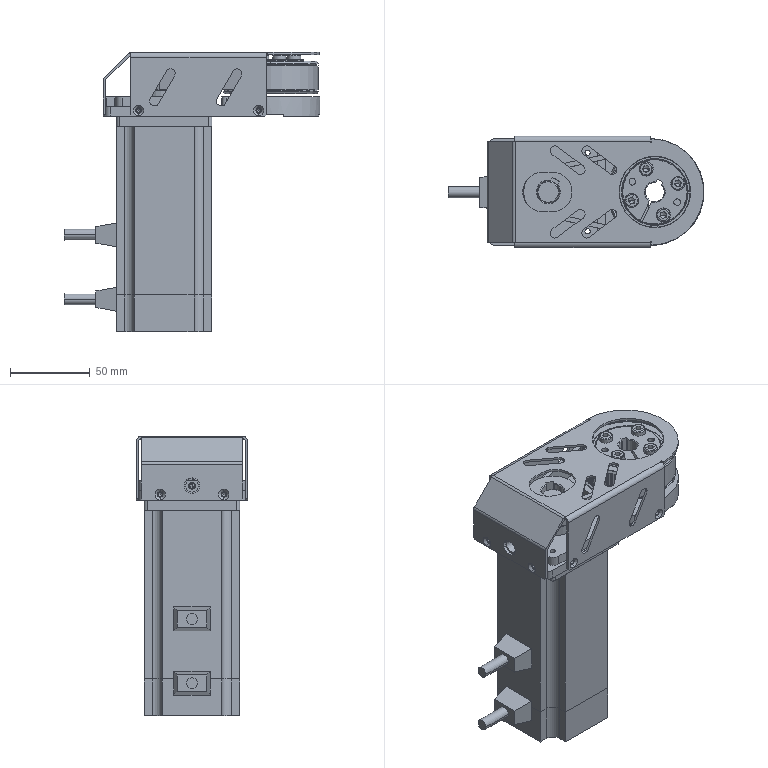Part | STEP file | Copy of CZ002-400W side link 2:1(K60)^K50A-1H20-S(formula driven)-L300-motor left- | 19 solids | 1055 faces | box 161.001 x 70 x 175.5 mm | volume 580294 mm3 | cylinder 681 | plane 254 | cone 102 | spline 18 | commonest cylinder face diameters 0.6 x224 1.82 x132 56.53 x60 6 x34 28 x32 5.5 x28